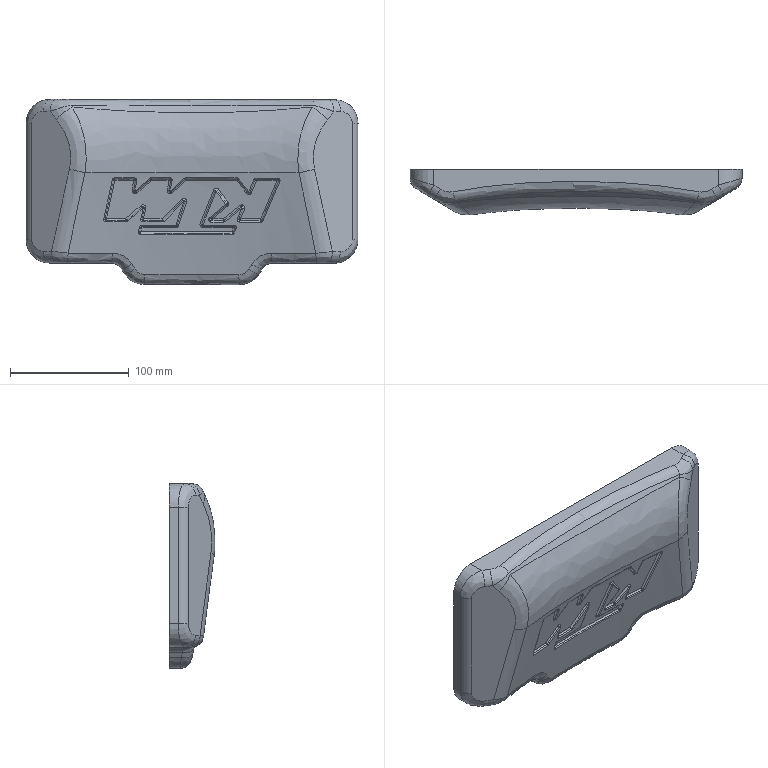Part | SolidWorks | features BaseBody 1 | 1 solid | 197 faces | box 280.077 x 38.808 x 156.126 mm | volume 1095780 mm3 | spline 141 | cylinder 33 | sphere 12 | plane 11 | commonest cylinder face diameters 2 x10 20 x8 40 x6 3 x5 2.001 x2 2.999 x2